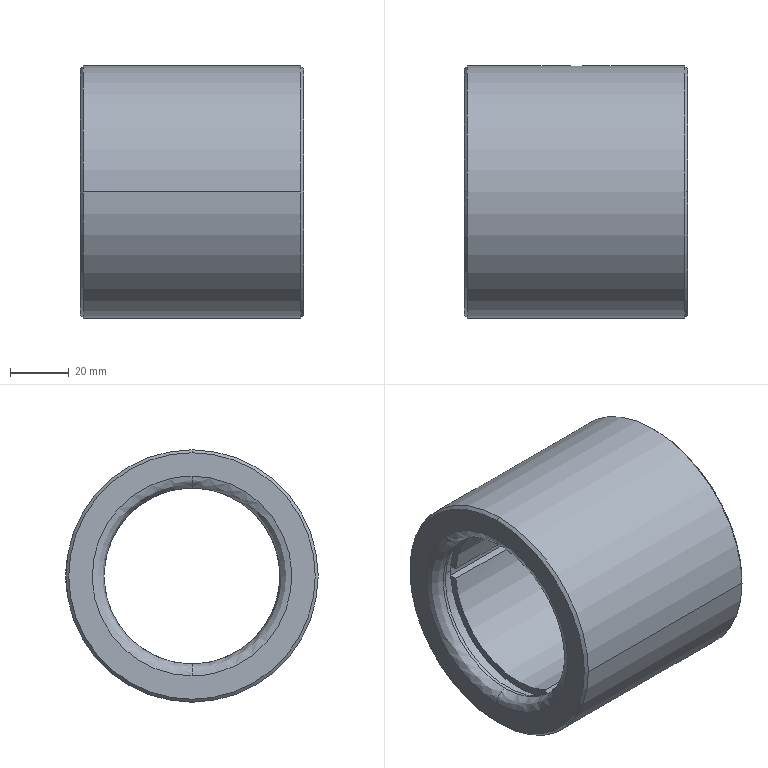Part | SolidWorks | features BaseBody 1 | 1 solid | 57 faces | box 76 x 86 x 86 mm | volume 218570 mm3 | plane 34 | cylinder 15 | cone 6 | spline 2 | commonest cylinder face diameters 60 x7 65 x4 6 x2 86 x2